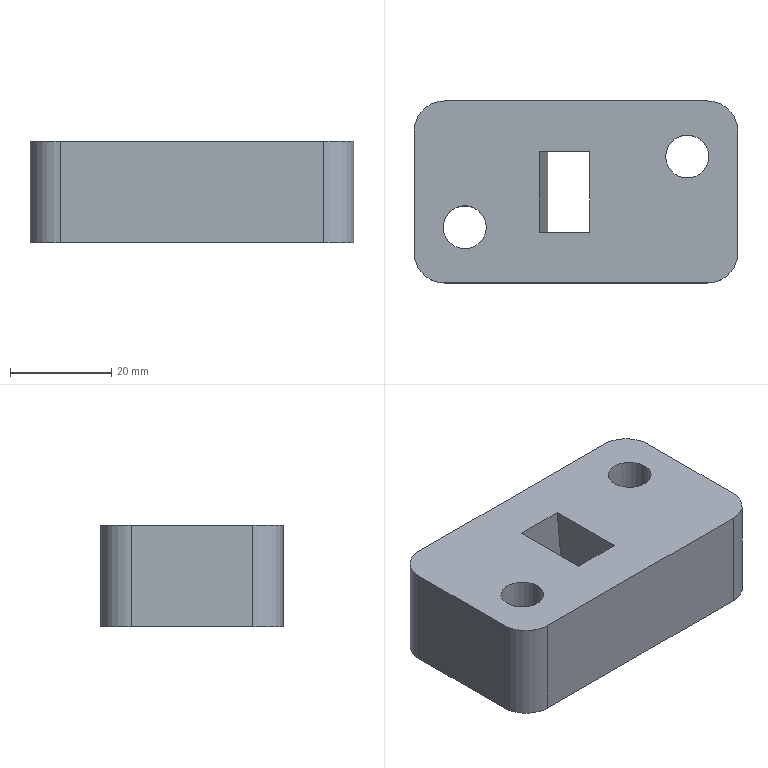Part | STEP file | solid 103 | 1 solid | 27 faces | box 64 x 36 x 20 mm | volume 38230 mm3 | plane 15 | cylinder 8 | other 4 | commonest cylinder face diameters 12 x4 8.5 x2 14 x2